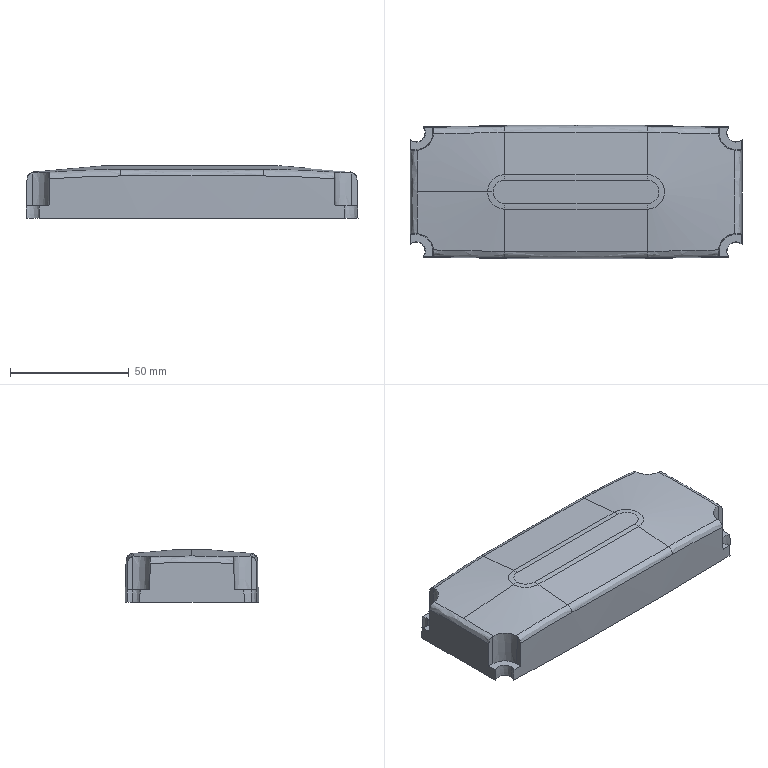Part | SolidWorks | features BaseBody 1 | 1 solid | 47 faces | box 140.075 x 56.575 x 22.3 mm | volume 156798 mm3 | plane 18 | cone 16 | spline 11 | cylinder 2 | commonest cylinder face diameters 55.6 x2